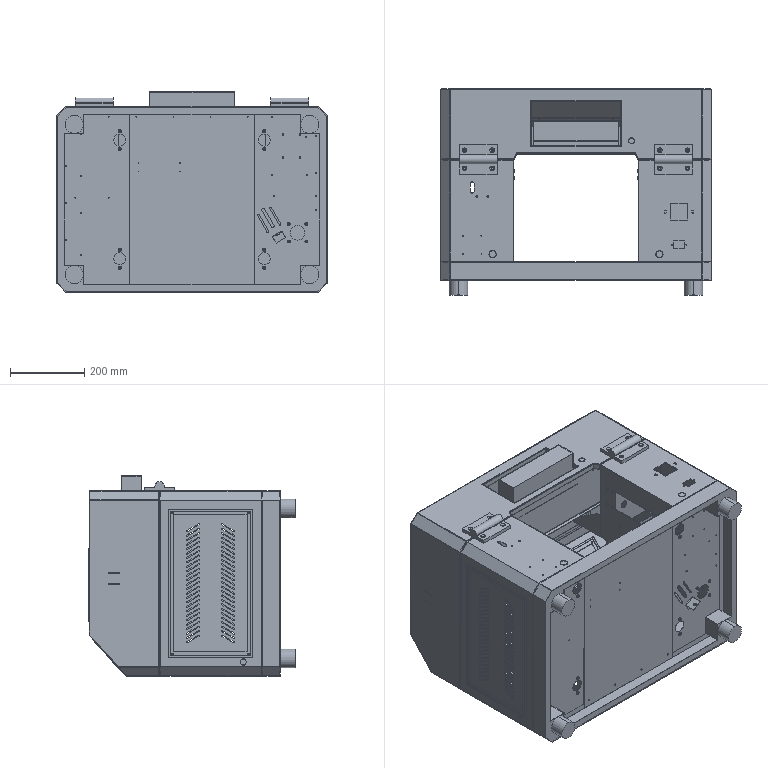Part | SolidWorks | 19 solids | 1957 faces | box 730 x 556.8 x 540 mm | volume 4115428 mm3 | cylinder 1092 | plane 753 | cone 52 | sphere 36 | spline 16 | torus 8 | commonest cylinder face diameters 3 x312 2.5 x182 3.3 x92 4 x71 4.2 x58 5 x42